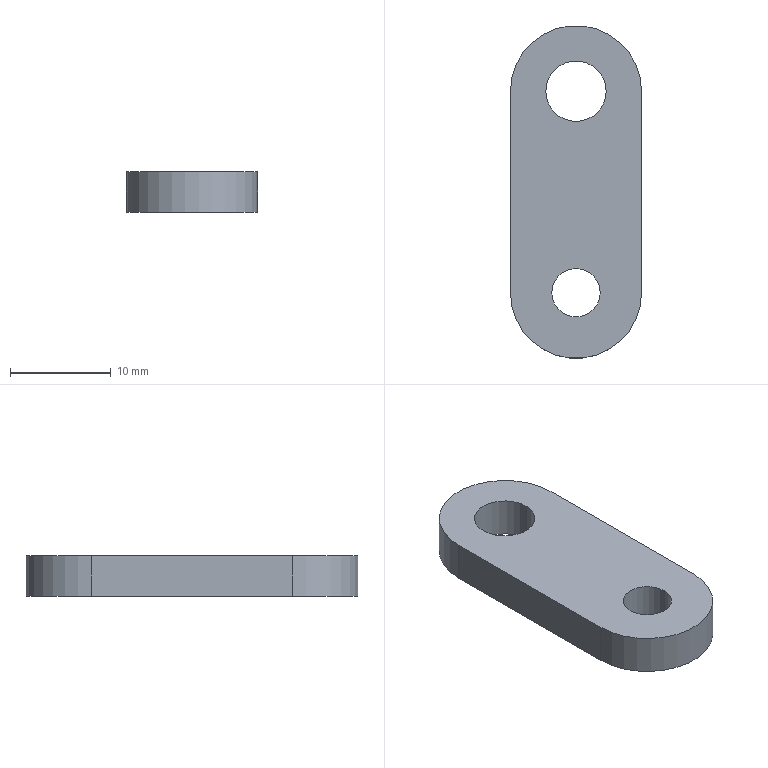Part | SolidWorks | features Extrusion 1 | 1 solid | 10 faces | box 13 x 33 x 4 mm | volume 1385 mm3 | cylinder 6 | plane 4 | commonest cylinder face diameters 4.8 x2 6 x2 13 x2
STEP:
#1=CARTESIAN_POINT('',(-2.4,-20.,4.));
#2=VERTEX_POINT('',#1);
#3=CARTESIAN_POINT('',(2.4,-20.,4.));
#4=VERTEX_POINT('',#3);
#5=CARTESIAN_POINT('',(0.,-20.,4.));
#6=DIRECTION('',(0.,0.,1.));
#7=DIRECTION('',(1.,0.,0.));
#8=AXIS2_PLACEMENT_3D('',#5,#6,#7);
#9=CIRCLE('',#8,2.4);
#10=EDGE_CURVE('',#2,#4,#9,.T.);
#11=ORIENTED_EDGE('',*,*,#10,.T.);
#12=CARTESIAN_POINT('',(2.4,-20.,0.));
#13=VERTEX_POINT('',#12);
#14=CARTESIAN_POINT('',(2.4,-20.,4.));
#15=DIRECTION('',(0.,0.,-1.));
#16=VECTOR('',#15,1000.);
#17=LINE('',#14,#16);
#18=EDGE_CURVE('',#4,#13,#17,.T.);
#19=ORIENTED_EDGE('',*,*,#18,.T.);
#20=CARTESIAN_POINT('',(-2.4,-20.,0.));
#21=VERTEX_POINT('',#20);
#22=CARTESIAN_POINT('',(0.,-20.,0.));
#23=DIRECTION('',(0.,0.,1.));
#24=DIRECTION('',(1.,0.,0.));
#25=AXIS2_PLACEMENT_3D('',#22,#23,#24);
#26=CIRCLE('',#25,2.4);
#27=EDGE_CURVE('',#21,#13,#26,.T.);
#28=ORIENTED_EDGE('',*,*,#27,.F.);
#29=CARTESIAN_POINT('',(-2.4,-20.,4.));
#30=DIRECTION('',(0.,0.,-1.));
#31=VECTOR('',#30,1000.);
#32=LINE('',#29,#31);
#33=EDGE_CURVE('',#2,#21,#32,.T.);
#34=ORIENTED_EDGE('',*,*,#33,.F.);
#35=EDGE_LOOP('',(#11,#19,#28,#34));
#36=FACE_OUTER_BOUND('',#35,.T.);
#37=CARTESIAN_POINT('',(0.,-20.,4.));
#38=DIRECTION('',(0.,0.,-1.));
#39=DIRECTION('',(-1.,0.,0.));
#40=AXIS2_PLACEMENT_3D('',#37,#38,#39);
#41=CYLINDRICAL_SURFACE('',#40,2.4);
#42=ADVANCED_FACE('',(#36),#41,.F.);
#43=CARTESIAN_POINT('',(-3.,0.,4.));
#44=VERTEX_POINT('',#43);
#45=CARTESIAN_POINT('',(3.,0.,4.));
#46=VERTEX_POINT('',#45);
#47=CARTESIAN_POINT('',(0.,0.,4.));
#48=DIRECTION('',(0.,0.,1.));
#49=DIRECTION('',(1.,0.,0.));
#50=AXIS2_PLACEMENT_3D('',#47,#48,#49);
#51=CIRCLE('',#50,3.);
#52=EDGE_CURVE('',#44,#46,#51,.T.);
#53=ORIENTED_EDGE('',*,*,#52,.T.);
#54=CARTESIAN_POINT('',(3.,0.,0.));
#55=VERTEX_POINT('',#54);
#56=CARTESIAN_POINT('',(3.,0.,4.));
#57=DIRECTION('',(0.,0.,-1.));
#58=VECTOR('',#57,1000.);
#59=LINE('',#56,#58);
#60=EDGE_CURVE('',#46,#55,#59,.T.);
#61=ORIENTED_EDGE('',*,*,#60,.T.);
#62=CARTESIAN_POINT('',(-3.,0.,0.));
#63=VERTEX_POINT('',#62);
#64=CARTESIAN_POINT('',(0.,0.,0.));
#65=DIRECTION('',(0.,0.,1.));
#66=DIRECTION('',(1.,0.,0.));
#67=AXIS2_PLACEMENT_3D('',#64,#65,#66);
#68=CIRCLE('',#67,3.);
#69=EDGE_CURVE('',#63,#55,#68,.T.);
#70=ORIENTED_EDGE('',*,*,#69,.F.);
#71=CARTESIAN_POINT('',(-3.,0.,4.));
#72=DIRECTION('',(0.,0.,-1.));
#73=VECTOR('',#72,1000.);
#74=LINE('',#71,#73);
#75=EDGE_CURVE('',#44,#63,#74,.T.);
#76=ORIENTED_EDGE('',*,*,#75,.F.);
#77=EDGE_LOOP('',(#53,#61,#70,#76));
#78=FACE_OUTER_BOUND('',#77,.T.);
#79=CARTESIAN_POINT('',(0.,0.,4.));
#80=DIRECTION('',(0.,0.,-1.));
#81=DIRECTION('',(-1.,0.,0.));
#82=AXIS2_PLACEMENT_3D('',#79,#80,#81);
#83=CYLINDRICAL_SURFACE('',#82,3.);
#84=ADVANCED_FACE('',(#78),#83,.F.);
#85=ORIENTED_EDGE('',*,*,#52,.F.);
#86=CARTESIAN_POINT('',(0.,0.,4.));
#87=DIRECTION('',(0.,0.,1.));
#88=DIRECTION('',(1.,0.,0.));
#89=AXIS2_PLACEMENT_3D('',#86,#87,#88);
#90=CIRCLE('',#89,3.);
#91=EDGE_CURVE('',#46,#44,#90,.T.);
#92=ORIENTED_EDGE('',*,*,#91,.F.);
#93=EDGE_LOOP('',(#85,#92));
#94=FACE_BOUND('',#93,.T.);
#95=CARTESIAN_POINT('',(6.5,0.,4.));
#96=VERTEX_POINT('',#95);
#97=CARTESIAN_POINT('',(-6.5,0.,4.));
#98=VERTEX_POINT('',#97);
#99=CARTESIAN_POINT('',(0.,0.,4.));
#100=DIRECTION('',(0.,0.,1.));
#101=DIRECTION('',(1.,0.,0.));
#102=AXIS2_PLACEMENT_3D('',#99,#100,#101);
#103=CIRCLE('',#102,6.5);
#104=EDGE_CURVE('',#96,#98,#103,.T.);
#105=ORIENTED_EDGE('',*,*,#104,.T.);
#106=CARTESIAN_POINT('',(-6.5,-20.,4.));
#107=VERTEX_POINT('',#106);
#108=CARTESIAN_POINT('',(-6.5,-20.,4.));
#109=DIRECTION('',(0.,-1.,0.));
#110=VECTOR('',#109,1000.);
#111=LINE('',#108,#110);
#112=EDGE_CURVE('',#98,#107,#111,.T.);
#113=ORIENTED_EDGE('',*,*,#112,.T.);
#114=CARTESIAN_POINT('',(6.5,-20.,4.));
#115=VERTEX_POINT('',#114);
#116=CARTESIAN_POINT('',(0.,-20.,4.));
#117=DIRECTION('',(0.,0.,1.));
#118=DIRECTION('',(1.,0.,0.));
#119=AXIS2_PLACEMENT_3D('',#116,#117,#118);
#120=CIRCLE('',#119,6.5);
#121=EDGE_CURVE('',#107,#115,#120,.T.);
#122=ORIENTED_EDGE('',*,*,#121,.T.);
#123=CARTESIAN_POINT('',(6.5,0.,4.));
#124=DIRECTION('',(0.,1.,0.));
#125=VECTOR('',#124,1000.);
#126=LINE('',#123,#125);
#127=EDGE_CURVE('',#115,#96,#126,.T.);
#128=ORIENTED_EDGE('',*,*,#127,.T.);
#129=EDGE_LOOP('',(#105,#113,#122,#128));
#130=FACE_OUTER_BOUND('',#129,.T.);
#131=ORIENTED_EDGE('',*,*,#10,.F.);
#132=CARTESIAN_POINT('',(0.,-20.,4.));
#133=DIRECTION('',(0.,0.,1.));
#134=DIRECTION('',(1.,0.,0.));
#135=AXIS2_PLACEMENT_3D('',#132,#133,#134);
#136=CIRCLE('',#135,2.4);
#137=EDGE_CURVE('',#4,#2,#136,.T.);
#138=ORIENTED_EDGE('',*,*,#137,.F.);
#139=EDGE_LOOP('',(#131,#138));
#140=FACE_BOUND('',#139,.T.);
#141=CARTESIAN_POINT('',(0.,0.,4.));
#142=DIRECTION('',(0.,0.,1.));
#143=DIRECTION('',(1.,0.,0.));
#144=AXIS2_PLACEMENT_3D('',#141,#142,#143);
#145=PLANE('',#144);
#146=ADVANCED_FACE('',(#94,#130,#140),#145,.T.);
#147=ORIENTED_EDGE('',*,*,#69,.T.);
#148=CARTESIAN_POINT('',(0.,0.,0.));
#149=DIRECTION('',(0.,0.,1.));
#150=DIRECTION('',(1.,0.,0.));
#151=AXIS2_PLACEMENT_3D('',#148,#149,#150);
#152=CIRCLE('',#151,3.);
#153=EDGE_CURVE('',#55,#63,#152,.T.);
#154=ORIENTED_EDGE('',*,*,#153,.T.);
#155=EDGE_LOOP('',(#147,#154));
#156=FACE_BOUND('',#155,.T.);
#157=CARTESIAN_POINT('',(6.5,0.,0.));
#158=VERTEX_POINT('',#157);
#159=CARTESIAN_POINT('',(-6.5,0.,0.));
#160=VERTEX_POINT('',#159);
#161=CARTESIAN_POINT('',(0.,0.,0.));
#162=DIRECTION('',(0.,0.,1.));
#163=DIRECTION('',(1.,0.,0.));
#164=AXIS2_PLACEMENT_3D('',#161,#162,#163);
#165=CIRCLE('',#164,6.5);
#166=EDGE_CURVE('',#158,#160,#165,.T.);
#167=ORIENTED_EDGE('',*,*,#166,.F.);
#168=CARTESIAN_POINT('',(6.5,-20.,0.));
#169=VERTEX_POINT('',#168);
#170=CARTESIAN_POINT('',(6.5,0.,0.));
#171=DIRECTION('',(0.,1.,0.));
#172=VECTOR('',#171,1000.);
#173=LINE('',#170,#172);
#174=EDGE_CURVE('',#169,#158,#173,.T.);
#175=ORIENTED_EDGE('',*,*,#174,.F.);
#176=CARTESIAN_POINT('',(-6.5,-20.,0.));
#177=VERTEX_POINT('',#176);
#178=CARTESIAN_POINT('',(0.,-20.,0.));
#179=DIRECTION('',(0.,0.,1.));
#180=DIRECTION('',(1.,0.,0.));
#181=AXIS2_PLACEMENT_3D('',#178,#179,#180);
#182=CIRCLE('',#181,6.5);
#183=EDGE_CURVE('',#177,#169,#182,.T.);
#184=ORIENTED_EDGE('',*,*,#183,.F.);
#185=CARTESIAN_POINT('',(-6.5,-20.,0.));
#186=DIRECTION('',(0.,-1.,0.));
#187=VECTOR('',#186,1000.);
#188=LINE('',#185,#187);
#189=EDGE_CURVE('',#160,#177,#188,.T.);
#190=ORIENTED_EDGE('',*,*,#189,.F.);
#191=EDGE_LOOP('',(#167,#175,#184,#190));
#192=FACE_OUTER_BOUND('',#191,.T.);
#193=ORIENTED_EDGE('',*,*,#27,.T.);
#194=CARTESIAN_POINT('',(0.,-20.,0.));
#195=DIRECTION('',(0.,0.,1.));
#196=DIRECTION('',(1.,0.,0.));
#197=AXIS2_PLACEMENT_3D('',#194,#195,#196);
#198=CIRCLE('',#197,2.4);
#199=EDGE_CURVE('',#13,#21,#198,.T.);
#200=ORIENTED_EDGE('',*,*,#199,.T.);
#201=EDGE_LOOP('',(#193,#200));
#202=FACE_BOUND('',#201,.T.);
#203=CARTESIAN_POINT('',(0.,0.,0.));
#204=DIRECTION('',(0.,0.,1.));
#205=DIRECTION('',(1.,0.,0.));
#206=AXIS2_PLACEMENT_3D('',#203,#204,#205);
#207=PLANE('',#206);
#208=ADVANCED_FACE('',(#156,#192,#202),#207,.F.);
#209=ORIENTED_EDGE('',*,*,#166,.T.);
#210=CARTESIAN_POINT('',(-6.5,0.,4.));
#211=DIRECTION('',(0.,0.,-1.));
#212=VECTOR('',#211,1000.);
#213=LINE('',#210,#212);
#214=EDGE_CURVE('',#98,#160,#213,.T.);
#215=ORIENTED_EDGE('',*,*,#214,.F.);
#216=ORIENTED_EDGE('',*,*,#104,.F.);
#217=CARTESIAN_POINT('',(6.5,0.,4.));
#218=DIRECTION('',(0.,0.,-1.));
#219=VECTOR('',#218,1000.);
#220=LINE('',#217,#219);
#221=EDGE_CURVE('',#96,#158,#220,.T.);
#222=ORIENTED_EDGE('',*,*,#221,.T.);
#223=EDGE_LOOP('',(#209,#215,#216,#222));
#224=FACE_OUTER_BOUND('',#223,.T.);
#225=CARTESIAN_POINT('',(0.,0.,4.));
#226=DIRECTION('',(0.,0.,-1.));
#227=DIRECTION('',(-1.,0.,0.));
#228=AXIS2_PLACEMENT_3D('',#225,#226,#227);
#229=CYLINDRICAL_SURFACE('',#228,6.5);
#230=ADVANCED_FACE('',(#224),#229,.T.);
#231=ORIENTED_EDGE('',*,*,#189,.T.);
#232=CARTESIAN_POINT('',(-6.5,-20.,4.));
#233=DIRECTION('',(0.,0.,-1.));
#234=VECTOR('',#233,1000.);
#235=LINE('',#232,#234);
#236=EDGE_CURVE('',#107,#177,#235,.T.);
#237=ORIENTED_EDGE('',*,*,#236,.F.);
#238=ORIENTED_EDGE('',*,*,#112,.F.);
#239=ORIENTED_EDGE('',*,*,#214,.T.);
#240=EDGE_LOOP('',(#231,#237,#238,#239));
#241=FACE_OUTER_BOUND('',#240,.T.);
#242=CARTESIAN_POINT('',(-6.5,-20.,4.));
#243=DIRECTION('',(1.,0.,0.));
#244=DIRECTION('',(0.,0.,-1.));
#245=AXIS2_PLACEMENT_3D('',#242,#243,#244);
#246=PLANE('',#245);
#247=ADVANCED_FACE('',(#241),#246,.F.);
#248=ORIENTED_EDGE('',*,*,#183,.T.);
#249=CARTESIAN_POINT('',(6.5,-20.,4.));
#250=DIRECTION('',(0.,0.,-1.));
#251=VECTOR('',#250,1000.);
#252=LINE('',#249,#251);
#253=EDGE_CURVE('',#115,#169,#252,.T.);
#254=ORIENTED_EDGE('',*,*,#253,.F.);
#255=ORIENTED_EDGE('',*,*,#121,.F.);
#256=ORIENTED_EDGE('',*,*,#236,.T.);
#257=EDGE_LOOP('',(#248,#254,#255,#256));
#258=FACE_OUTER_BOUND('',#257,.T.);
#259=CARTESIAN_POINT('',(0.,-20.,4.));
#260=DIRECTION('',(0.,0.,-1.));
#261=DIRECTION('',(-1.,0.,0.));
#262=AXIS2_PLACEMENT_3D('',#259,#260,#261);
#263=CYLINDRICAL_SURFACE('',#262,6.5);
#264=ADVANCED_FACE('',(#258),#263,.T.);
#265=ORIENTED_EDGE('',*,*,#174,.T.);
#266=ORIENTED_EDGE('',*,*,#221,.F.);
#267=ORIENTED_EDGE('',*,*,#127,.F.);
#268=ORIENTED_EDGE('',*,*,#253,.T.);
#269=EDGE_LOOP('',(#265,#266,#267,#268));
#270=FACE_OUTER_BOUND('',#269,.T.);
#271=CARTESIAN_POINT('',(6.5,0.,4.));
#272=DIRECTION('',(-1.,0.,0.));
#273=DIRECTION('',(0.,0.,1.));
#274=AXIS2_PLACEMENT_3D('',#271,#272,#273);
#275=PLANE('',#274);
#276=ADVANCED_FACE('',(#270),#275,.F.);
#277=ORIENTED_EDGE('',*,*,#60,.F.);
#278=ORIENTED_EDGE('',*,*,#91,.T.);
#279=ORIENTED_EDGE('',*,*,#75,.T.);
#280=ORIENTED_EDGE('',*,*,#153,.F.);
#281=EDGE_LOOP('',(#277,#278,#279,#280));
#282=FACE_OUTER_BOUND('',#281,.T.);
#283=CARTESIAN_POINT('',(0.,0.,4.));
#284=DIRECTION('',(0.,0.,-1.));
#285=DIRECTION('',(-1.,0.,0.));
#286=AXIS2_PLACEMENT_3D('',#283,#284,#285);
#287=CYLINDRICAL_SURFACE('',#286,3.);
#288=ADVANCED_FACE('',(#282),#287,.F.);
#289=ORIENTED_EDGE('',*,*,#18,.F.);
#290=ORIENTED_EDGE('',*,*,#137,.T.);
#291=ORIENTED_EDGE('',*,*,#33,.T.);
#292=ORIENTED_EDGE('',*,*,#199,.F.);
#293=EDGE_LOOP('',(#289,#290,#291,#292));
#294=FACE_OUTER_BOUND('',#293,.T.);
#295=CARTESIAN_POINT('',(0.,-20.,4.));
#296=DIRECTION('',(0.,0.,-1.));
#297=DIRECTION('',(-1.,0.,0.));
#298=AXIS2_PLACEMENT_3D('',#295,#296,#297);
#299=CYLINDRICAL_SURFACE('',#298,2.4);
#300=ADVANCED_FACE('',(#294),#299,.F.);
#301=CLOSED_SHELL('',(#42,#84,#146,#208,#230,#247,#264,#276,#288,#300));
#302=MANIFOLD_SOLID_BREP('',#301);
#303=CARTESIAN_POINT('',(0.,0.,0.));
#304=DIRECTION('',(0.,0.,1.));
#305=DIRECTION('',(1.,0.,0.));
#306=AXIS2_PLACEMENT_3D('',#303,#304,#305);
#307=(LENGTH_UNIT()NAMED_UNIT(*)SI_UNIT(.MILLI.,.METRE.));
#308=UNCERTAINTY_MEASURE_WITH_UNIT(LENGTH_MEASURE(0.00001),#307,'','');
#309=(NAMED_UNIT(*)PLANE_ANGLE_UNIT()SI_UNIT($,.RADIAN.));
#310=(NAMED_UNIT(*)SI_UNIT($,.STERADIAN.)SOLID_ANGLE_UNIT());
#311=(GEOMETRIC_REPRESENTATION_CONTEXT(3)GLOBAL_UNCERTAINTY_ASSIGNED_CONTEXT((#308))GLOBAL_UNIT_ASSIGNED_CONTEXT((#307,#309,#310))REPRESENTATION_CONTEXT('',''));
#312=ADVANCED_BREP_SHAPE_REPRESENTATION('',(#302,#306),#311);